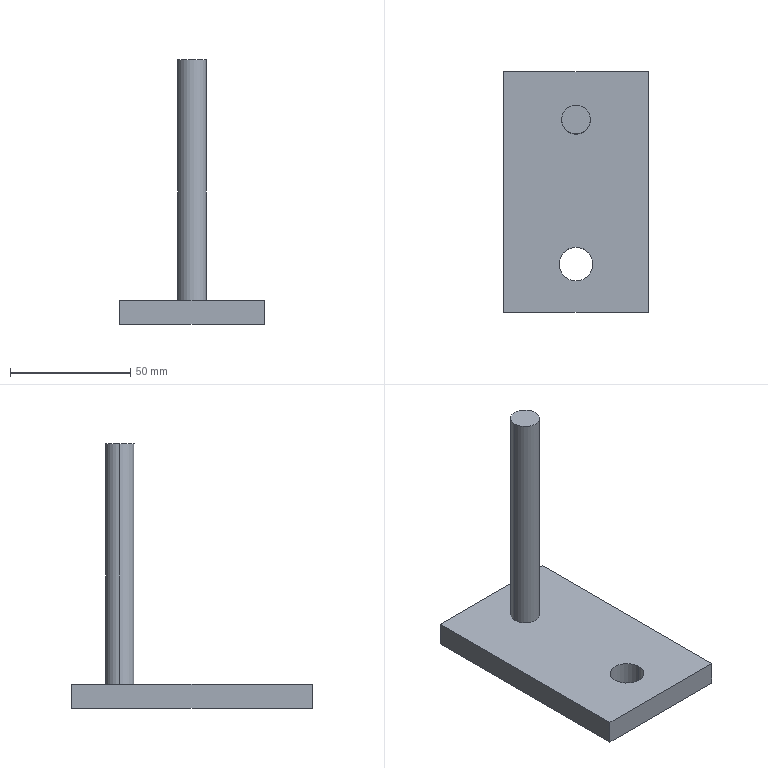Part | SolidWorks | features Extrusion 1, ICE 1 | 1 solid | 11 faces | box 60 x 100 x 110 mm | volume 69770 mm3 | plane 7 | cylinder 4 | commonest cylinder face diameters 12 x2 14 x2
STEP:
#1=CARTESIAN_POINT('',(6.,30.,110.));
#2=VERTEX_POINT('',#1);
#3=CARTESIAN_POINT('',(-6.,30.,110.));
#4=VERTEX_POINT('',#3);
#5=CARTESIAN_POINT('',(0.,30.,110.));
#6=DIRECTION('',(0.,0.,1.));
#7=DIRECTION('',(1.,0.,0.));
#8=AXIS2_PLACEMENT_3D('',#5,#6,#7);
#9=CIRCLE('',#8,6.);
#10=EDGE_CURVE('',#2,#4,#9,.T.);
#11=ORIENTED_EDGE('',*,*,#10,.F.);
#12=CARTESIAN_POINT('',(6.,30.,10.));
#13=VERTEX_POINT('',#12);
#14=CARTESIAN_POINT('',(6.,30.,110.));
#15=DIRECTION('',(0.,0.,-1.));
#16=VECTOR('',#15,1000.);
#17=LINE('',#14,#16);
#18=EDGE_CURVE('',#2,#13,#17,.T.);
#19=ORIENTED_EDGE('',*,*,#18,.T.);
#20=CARTESIAN_POINT('',(-6.,30.,10.));
#21=VERTEX_POINT('',#20);
#22=CARTESIAN_POINT('',(0.,30.,10.));
#23=DIRECTION('',(0.,0.,1.));
#24=DIRECTION('',(-1.,0.,0.));
#25=AXIS2_PLACEMENT_3D('',#22,#23,#24);
#26=CIRCLE('',#25,6.);
#27=EDGE_CURVE('',#13,#21,#26,.T.);
#28=ORIENTED_EDGE('',*,*,#27,.T.);
#29=CARTESIAN_POINT('',(-6.,30.,110.));
#30=DIRECTION('',(0.,0.,-1.));
#31=VECTOR('',#30,1000.);
#32=LINE('',#29,#31);
#33=EDGE_CURVE('',#4,#21,#32,.T.);
#34=ORIENTED_EDGE('',*,*,#33,.F.);
#35=EDGE_LOOP('',(#11,#19,#28,#34));
#36=FACE_OUTER_BOUND('',#35,.T.);
#37=CARTESIAN_POINT('',(0.,30.,110.));
#38=DIRECTION('',(0.,0.,-1.));
#39=DIRECTION('',(-1.,0.,0.));
#40=AXIS2_PLACEMENT_3D('',#37,#38,#39);
#41=CYLINDRICAL_SURFACE('',#40,6.);
#42=ADVANCED_FACE('',(#36),#41,.T.);
#43=CARTESIAN_POINT('',(-7.,-30.,10.));
#44=VERTEX_POINT('',#43);
#45=CARTESIAN_POINT('',(7.,-30.,10.));
#46=VERTEX_POINT('',#45);
#47=CARTESIAN_POINT('',(0.,-30.,10.));
#48=DIRECTION('',(0.,0.,1.));
#49=DIRECTION('',(1.,0.,0.));
#50=AXIS2_PLACEMENT_3D('',#47,#48,#49);
#51=CIRCLE('',#50,7.);
#52=EDGE_CURVE('',#44,#46,#51,.T.);
#53=ORIENTED_EDGE('',*,*,#52,.T.);
#54=CARTESIAN_POINT('',(7.,-30.,0.));
#55=VERTEX_POINT('',#54);
#56=CARTESIAN_POINT('',(7.,-30.,10.));
#57=DIRECTION('',(0.,0.,-1.));
#58=VECTOR('',#57,1000.);
#59=LINE('',#56,#58);
#60=EDGE_CURVE('',#46,#55,#59,.T.);
#61=ORIENTED_EDGE('',*,*,#60,.T.);
#62=CARTESIAN_POINT('',(-7.,-30.,0.));
#63=VERTEX_POINT('',#62);
#64=CARTESIAN_POINT('',(0.,-30.,0.));
#65=DIRECTION('',(0.,0.,1.));
#66=DIRECTION('',(1.,0.,0.));
#67=AXIS2_PLACEMENT_3D('',#64,#65,#66);
#68=CIRCLE('',#67,7.);
#69=EDGE_CURVE('',#63,#55,#68,.T.);
#70=ORIENTED_EDGE('',*,*,#69,.F.);
#71=CARTESIAN_POINT('',(-7.,-30.,10.));
#72=DIRECTION('',(0.,0.,-1.));
#73=VECTOR('',#72,1000.);
#74=LINE('',#71,#73);
#75=EDGE_CURVE('',#44,#63,#74,.T.);
#76=ORIENTED_EDGE('',*,*,#75,.F.);
#77=EDGE_LOOP('',(#53,#61,#70,#76));
#78=FACE_OUTER_BOUND('',#77,.T.);
#79=CARTESIAN_POINT('',(0.,-30.,10.));
#80=DIRECTION('',(0.,0.,-1.));
#81=DIRECTION('',(-1.,0.,0.));
#82=AXIS2_PLACEMENT_3D('',#79,#80,#81);
#83=CYLINDRICAL_SURFACE('',#82,7.);
#84=ADVANCED_FACE('',(#78),#83,.F.);
#85=CARTESIAN_POINT('',(0.,30.,10.));
#86=DIRECTION('',(0.,0.,1.));
#87=DIRECTION('',(-1.,0.,0.));
#88=AXIS2_PLACEMENT_3D('',#85,#86,#87);
#89=CIRCLE('',#88,6.);
#90=EDGE_CURVE('',#21,#13,#89,.T.);
#91=ORIENTED_EDGE('',*,*,#90,.F.);
#92=ORIENTED_EDGE('',*,*,#27,.F.);
#93=EDGE_LOOP('',(#91,#92));
#94=FACE_BOUND('',#93,.T.);
#95=CARTESIAN_POINT('',(30.,-50.,10.));
#96=VERTEX_POINT('',#95);
#97=CARTESIAN_POINT('',(30.,50.,10.));
#98=VERTEX_POINT('',#97);
#99=CARTESIAN_POINT('',(30.,-50.,10.));
#100=DIRECTION('',(0.,1.,0.));
#101=VECTOR('',#100,1000.);
#102=LINE('',#99,#101);
#103=EDGE_CURVE('',#96,#98,#102,.T.);
#104=ORIENTED_EDGE('',*,*,#103,.T.);
#105=CARTESIAN_POINT('',(-30.,50.,10.));
#106=VERTEX_POINT('',#105);
#107=CARTESIAN_POINT('',(-30.,50.,10.));
#108=DIRECTION('',(-1.,0.,0.));
#109=VECTOR('',#108,1000.);
#110=LINE('',#107,#109);
#111=EDGE_CURVE('',#98,#106,#110,.T.);
#112=ORIENTED_EDGE('',*,*,#111,.T.);
#113=CARTESIAN_POINT('',(-30.,-50.,10.));
#114=VERTEX_POINT('',#113);
#115=CARTESIAN_POINT('',(-30.,-50.,10.));
#116=DIRECTION('',(0.,-1.,0.));
#117=VECTOR('',#116,1000.);
#118=LINE('',#115,#117);
#119=EDGE_CURVE('',#106,#114,#118,.T.);
#120=ORIENTED_EDGE('',*,*,#119,.T.);
#121=CARTESIAN_POINT('',(-30.,-50.,10.));
#122=DIRECTION('',(1.,0.,0.));
#123=VECTOR('',#122,1000.);
#124=LINE('',#121,#123);
#125=EDGE_CURVE('',#114,#96,#124,.T.);
#126=ORIENTED_EDGE('',*,*,#125,.T.);
#127=EDGE_LOOP('',(#104,#112,#120,#126));
#128=FACE_OUTER_BOUND('',#127,.T.);
#129=ORIENTED_EDGE('',*,*,#52,.F.);
#130=CARTESIAN_POINT('',(0.,-30.,10.));
#131=DIRECTION('',(0.,0.,1.));
#132=DIRECTION('',(1.,0.,0.));
#133=AXIS2_PLACEMENT_3D('',#130,#131,#132);
#134=CIRCLE('',#133,7.);
#135=EDGE_CURVE('',#46,#44,#134,.T.);
#136=ORIENTED_EDGE('',*,*,#135,.F.);
#137=EDGE_LOOP('',(#129,#136));
#138=FACE_BOUND('',#137,.T.);
#139=CARTESIAN_POINT('',(0.,0.,10.));
#140=DIRECTION('',(0.,0.,-1.));
#141=DIRECTION('',(-1.,0.,0.));
#142=AXIS2_PLACEMENT_3D('',#139,#140,#141);
#143=PLANE('',#142);
#144=ADVANCED_FACE('',(#94,#128,#138),#143,.F.);
#145=CARTESIAN_POINT('',(30.,-50.,0.));
#146=VERTEX_POINT('',#145);
#147=CARTESIAN_POINT('',(30.,50.,0.));
#148=VERTEX_POINT('',#147);
#149=CARTESIAN_POINT('',(30.,-50.,0.));
#150=DIRECTION('',(0.,1.,0.));
#151=VECTOR('',#150,1000.);
#152=LINE('',#149,#151);
#153=EDGE_CURVE('',#146,#148,#152,.T.);
#154=ORIENTED_EDGE('',*,*,#153,.F.);
#155=CARTESIAN_POINT('',(-30.,-50.,0.));
#156=VERTEX_POINT('',#155);
#157=CARTESIAN_POINT('',(-30.,-50.,0.));
#158=DIRECTION('',(1.,0.,0.));
#159=VECTOR('',#158,1000.);
#160=LINE('',#157,#159);
#161=EDGE_CURVE('',#156,#146,#160,.T.);
#162=ORIENTED_EDGE('',*,*,#161,.F.);
#163=CARTESIAN_POINT('',(-30.,50.,0.));
#164=VERTEX_POINT('',#163);
#165=CARTESIAN_POINT('',(-30.,-50.,0.));
#166=DIRECTION('',(0.,-1.,0.));
#167=VECTOR('',#166,1000.);
#168=LINE('',#165,#167);
#169=EDGE_CURVE('',#164,#156,#168,.T.);
#170=ORIENTED_EDGE('',*,*,#169,.F.);
#171=CARTESIAN_POINT('',(-30.,50.,0.));
#172=DIRECTION('',(-1.,0.,0.));
#173=VECTOR('',#172,1000.);
#174=LINE('',#171,#173);
#175=EDGE_CURVE('',#148,#164,#174,.T.);
#176=ORIENTED_EDGE('',*,*,#175,.F.);
#177=EDGE_LOOP('',(#154,#162,#170,#176));
#178=FACE_OUTER_BOUND('',#177,.T.);
#179=ORIENTED_EDGE('',*,*,#69,.T.);
#180=CARTESIAN_POINT('',(0.,-30.,0.));
#181=DIRECTION('',(0.,0.,1.));
#182=DIRECTION('',(1.,0.,0.));
#183=AXIS2_PLACEMENT_3D('',#180,#181,#182);
#184=CIRCLE('',#183,7.);
#185=EDGE_CURVE('',#55,#63,#184,.T.);
#186=ORIENTED_EDGE('',*,*,#185,.T.);
#187=EDGE_LOOP('',(#179,#186));
#188=FACE_BOUND('',#187,.T.);
#189=CARTESIAN_POINT('',(0.,0.,0.));
#190=DIRECTION('',(0.,0.,-1.));
#191=DIRECTION('',(-1.,0.,0.));
#192=AXIS2_PLACEMENT_3D('',#189,#190,#191);
#193=PLANE('',#192);
#194=ADVANCED_FACE('',(#178,#188),#193,.T.);
#195=ORIENTED_EDGE('',*,*,#153,.T.);
#196=CARTESIAN_POINT('',(30.,50.,10.));
#197=DIRECTION('',(0.,0.,-1.));
#198=VECTOR('',#197,1000.);
#199=LINE('',#196,#198);
#200=EDGE_CURVE('',#98,#148,#199,.T.);
#201=ORIENTED_EDGE('',*,*,#200,.F.);
#202=ORIENTED_EDGE('',*,*,#103,.F.);
#203=CARTESIAN_POINT('',(30.,-50.,10.));
#204=DIRECTION('',(0.,0.,-1.));
#205=VECTOR('',#204,1000.);
#206=LINE('',#203,#205);
#207=EDGE_CURVE('',#96,#146,#206,.T.);
#208=ORIENTED_EDGE('',*,*,#207,.T.);
#209=EDGE_LOOP('',(#195,#201,#202,#208));
#210=FACE_OUTER_BOUND('',#209,.T.);
#211=CARTESIAN_POINT('',(30.,-50.,10.));
#212=DIRECTION('',(-1.,0.,0.));
#213=DIRECTION('',(0.,0.,1.));
#214=AXIS2_PLACEMENT_3D('',#211,#212,#213);
#215=PLANE('',#214);
#216=ADVANCED_FACE('',(#210),#215,.F.);
#217=ORIENTED_EDGE('',*,*,#175,.T.);
#218=CARTESIAN_POINT('',(-30.,50.,10.));
#219=DIRECTION('',(0.,0.,-1.));
#220=VECTOR('',#219,1000.);
#221=LINE('',#218,#220);
#222=EDGE_CURVE('',#106,#164,#221,.T.);
#223=ORIENTED_EDGE('',*,*,#222,.F.);
#224=ORIENTED_EDGE('',*,*,#111,.F.);
#225=ORIENTED_EDGE('',*,*,#200,.T.);
#226=EDGE_LOOP('',(#217,#223,#224,#225));
#227=FACE_OUTER_BOUND('',#226,.T.);
#228=CARTESIAN_POINT('',(-30.,50.,10.));
#229=DIRECTION('',(0.,-1.,0.));
#230=DIRECTION('',(0.,0.,-1.));
#231=AXIS2_PLACEMENT_3D('',#228,#229,#230);
#232=PLANE('',#231);
#233=ADVANCED_FACE('',(#227),#232,.F.);
#234=ORIENTED_EDGE('',*,*,#169,.T.);
#235=CARTESIAN_POINT('',(-30.,-50.,10.));
#236=DIRECTION('',(0.,0.,-1.));
#237=VECTOR('',#236,1000.);
#238=LINE('',#235,#237);
#239=EDGE_CURVE('',#114,#156,#238,.T.);
#240=ORIENTED_EDGE('',*,*,#239,.F.);
#241=ORIENTED_EDGE('',*,*,#119,.F.);
#242=ORIENTED_EDGE('',*,*,#222,.T.);
#243=EDGE_LOOP('',(#234,#240,#241,#242));
#244=FACE_OUTER_BOUND('',#243,.T.);
#245=CARTESIAN_POINT('',(-30.,-50.,10.));
#246=DIRECTION('',(1.,0.,0.));
#247=DIRECTION('',(0.,0.,-1.));
#248=AXIS2_PLACEMENT_3D('',#245,#246,#247);
#249=PLANE('',#248);
#250=ADVANCED_FACE('',(#244),#249,.F.);
#251=ORIENTED_EDGE('',*,*,#161,.T.);
#252=ORIENTED_EDGE('',*,*,#207,.F.);
#253=ORIENTED_EDGE('',*,*,#125,.F.);
#254=ORIENTED_EDGE('',*,*,#239,.T.);
#255=EDGE_LOOP('',(#251,#252,#253,#254));
#256=FACE_OUTER_BOUND('',#255,.T.);
#257=CARTESIAN_POINT('',(-30.,-50.,10.));
#258=DIRECTION('',(0.,1.,0.));
#259=DIRECTION('',(0.,0.,1.));
#260=AXIS2_PLACEMENT_3D('',#257,#258,#259);
#261=PLANE('',#260);
#262=ADVANCED_FACE('',(#256),#261,.F.);
#263=ORIENTED_EDGE('',*,*,#60,.F.);
#264=ORIENTED_EDGE('',*,*,#135,.T.);
#265=ORIENTED_EDGE('',*,*,#75,.T.);
#266=ORIENTED_EDGE('',*,*,#185,.F.);
#267=EDGE_LOOP('',(#263,#264,#265,#266));
#268=FACE_OUTER_BOUND('',#267,.T.);
#269=CARTESIAN_POINT('',(0.,-30.,10.));
#270=DIRECTION('',(0.,0.,-1.));
#271=DIRECTION('',(-1.,0.,0.));
#272=AXIS2_PLACEMENT_3D('',#269,#270,#271);
#273=CYLINDRICAL_SURFACE('',#272,7.);
#274=ADVANCED_FACE('',(#268),#273,.F.);
#275=ORIENTED_EDGE('',*,*,#18,.F.);
#276=CARTESIAN_POINT('',(0.,30.,110.));
#277=DIRECTION('',(0.,0.,1.));
#278=DIRECTION('',(1.,0.,0.));
#279=AXIS2_PLACEMENT_3D('',#276,#277,#278);
#280=CIRCLE('',#279,6.);
#281=EDGE_CURVE('',#4,#2,#280,.T.);
#282=ORIENTED_EDGE('',*,*,#281,.F.);
#283=ORIENTED_EDGE('',*,*,#33,.T.);
#284=ORIENTED_EDGE('',*,*,#90,.T.);
#285=EDGE_LOOP('',(#275,#282,#283,#284));
#286=FACE_OUTER_BOUND('',#285,.T.);
#287=CARTESIAN_POINT('',(0.,30.,110.));
#288=DIRECTION('',(0.,0.,-1.));
#289=DIRECTION('',(-1.,0.,0.));
#290=AXIS2_PLACEMENT_3D('',#287,#288,#289);
#291=CYLINDRICAL_SURFACE('',#290,6.);
#292=ADVANCED_FACE('',(#286),#291,.T.);
#293=ORIENTED_EDGE('',*,*,#281,.T.);
#294=ORIENTED_EDGE('',*,*,#10,.T.);
#295=EDGE_LOOP('',(#293,#294));
#296=FACE_OUTER_BOUND('',#295,.T.);
#297=CARTESIAN_POINT('',(0.,30.,110.));
#298=DIRECTION('',(0.,0.,1.));
#299=DIRECTION('',(1.,0.,0.));
#300=AXIS2_PLACEMENT_3D('',#297,#298,#299);
#301=PLANE('',#300);
#302=ADVANCED_FACE('',(#296),#301,.T.);
#303=CLOSED_SHELL('',(#42,#84,#144,#194,#216,#233,#250,#262,#274,#292,#302));
#304=MANIFOLD_SOLID_BREP('',#303);
#305=CARTESIAN_POINT('',(0.,0.,0.));
#306=DIRECTION('',(0.,0.,1.));
#307=DIRECTION('',(1.,0.,0.));
#308=AXIS2_PLACEMENT_3D('',#305,#306,#307);
#309=(LENGTH_UNIT()NAMED_UNIT(*)SI_UNIT(.MILLI.,.METRE.));
#310=UNCERTAINTY_MEASURE_WITH_UNIT(LENGTH_MEASURE(0.00001),#309,'','');
#311=(NAMED_UNIT(*)PLANE_ANGLE_UNIT()SI_UNIT($,.RADIAN.));
#312=(NAMED_UNIT(*)SI_UNIT($,.STERADIAN.)SOLID_ANGLE_UNIT());
#313=(GEOMETRIC_REPRESENTATION_CONTEXT(3)GLOBAL_UNCERTAINTY_ASSIGNED_CONTEXT((#310))GLOBAL_UNIT_ASSIGNED_CONTEXT((#309,#311,#312))REPRESENTATION_CONTEXT('',''));
#314=ADVANCED_BREP_SHAPE_REPRESENTATION('',(#304,#308),#313);